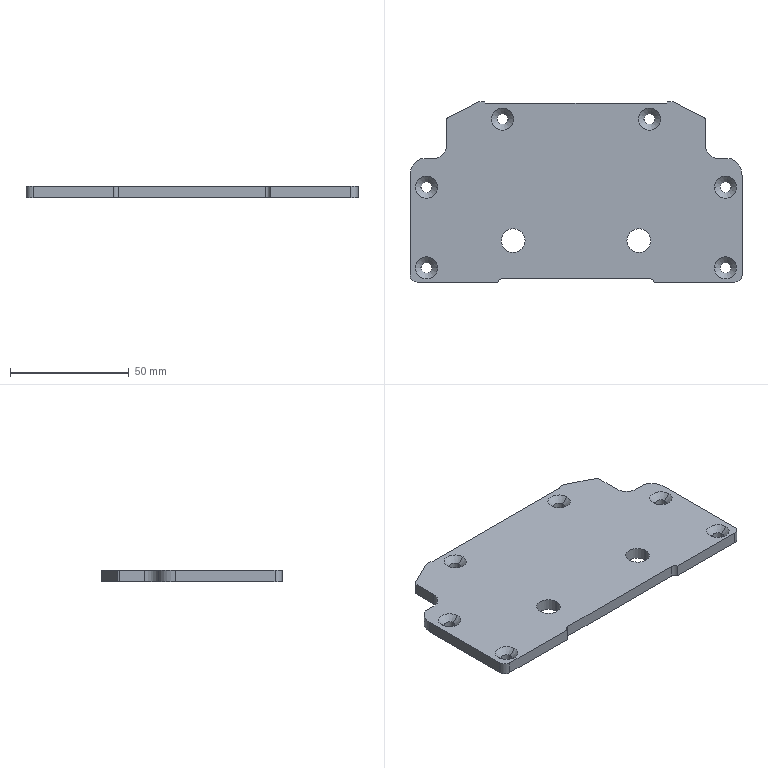Part | SolidWorks | features BaseBody 1 | 1 solid | 56 faces | box 140 x 76.005 x 5 mm | volume 46703 mm3 | cylinder 26 | plane 18 | cone 12 | commonest cylinder face diameters 4.5 x12 10 x4 2 x2 4 x2 6 x2 12 x2